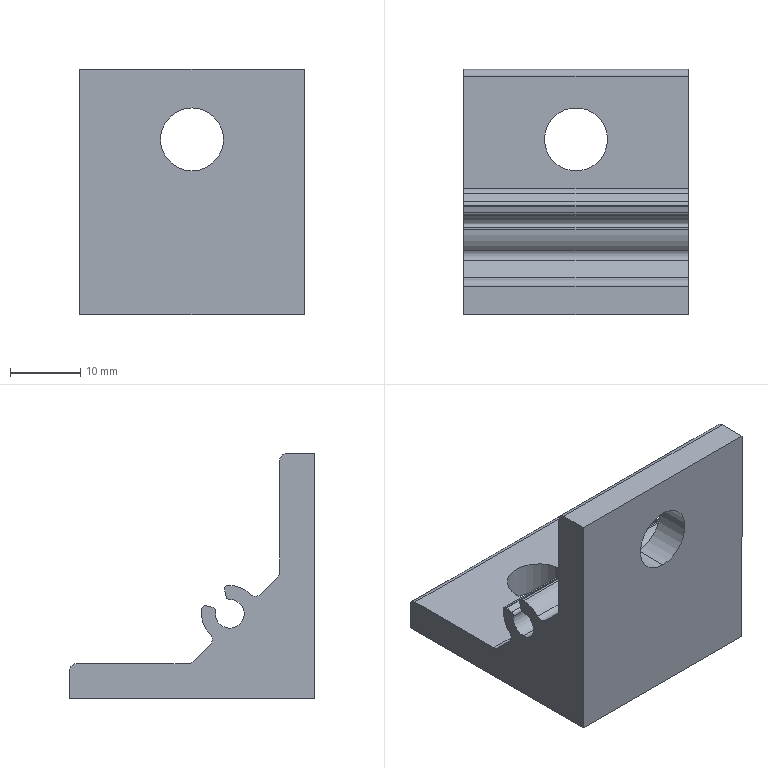Part | STEP file | HJLE-JJ90°-40_LE0724153021 | 1 solid | 33 faces | box 32 x 35 x 35 mm | volume 12807 mm3 | cylinder 21 | plane 12 | commonest cylinder face diameters 2 x6 1 x5 9 x4 4.1 x3 8.1 x3
STEP:
#1=CARTESIAN_POINT('',(0.,4.818,29.5));
#2=VERTEX_POINT('',#1);
#3=CARTESIAN_POINT('',(0.,4.818,20.5));
#4=VERTEX_POINT('',#3);
#5=CARTESIAN_POINT('',(0.,4.818,25.));
#6=DIRECTION('',(0.,-1.,0.));
#7=DIRECTION('',(0.,0.,-1.));
#8=AXIS2_PLACEMENT_3D('',#5,#6,#7);
#9=CIRCLE('',#8,4.5);
#10=EDGE_CURVE('',#2,#4,#9,.T.);
#11=ORIENTED_EDGE('',*,*,#10,.F.);
#12=CARTESIAN_POINT('',(0.,-0.182,29.5));
#13=VERTEX_POINT('',#12);
#14=CARTESIAN_POINT('',(0.,17.546,29.5));
#15=DIRECTION('',(0.,-1.,0.));
#16=VECTOR('',#15,1000.);
#17=LINE('',#14,#16);
#18=EDGE_CURVE('',#2,#13,#17,.T.);
#19=ORIENTED_EDGE('',*,*,#18,.T.);
#20=CARTESIAN_POINT('',(0.,-0.182,20.5));
#21=VERTEX_POINT('',#20);
#22=CARTESIAN_POINT('',(0.,-0.182,25.));
#23=DIRECTION('',(0.,-1.,0.));
#24=DIRECTION('',(0.,0.,-1.));
#25=AXIS2_PLACEMENT_3D('',#22,#23,#24);
#26=CIRCLE('',#25,4.5);
#27=EDGE_CURVE('',#13,#21,#26,.T.);
#28=ORIENTED_EDGE('',*,*,#27,.T.);
#29=CARTESIAN_POINT('',(0.,17.546,20.5));
#30=DIRECTION('',(0.,-1.,0.));
#31=VECTOR('',#30,1000.);
#32=LINE('',#29,#31);
#33=EDGE_CURVE('',#4,#21,#32,.T.);
#34=ORIENTED_EDGE('',*,*,#33,.F.);
#35=EDGE_LOOP('',(#11,#19,#28,#34));
#36=FACE_OUTER_BOUND('',#35,.T.);
#37=CARTESIAN_POINT('',(0.,17.546,25.));
#38=DIRECTION('',(0.,-1.,0.));
#39=DIRECTION('',(0.,0.,-1.));
#40=AXIS2_PLACEMENT_3D('',#37,#38,#39);
#41=CYLINDRICAL_SURFACE('',#40,4.5);
#42=ADVANCED_FACE('',(#36),#41,.F.);
#43=CARTESIAN_POINT('',(4.5,24.818,5.));
#44=VERTEX_POINT('',#43);
#45=CARTESIAN_POINT('',(-4.5,24.818,5.));
#46=VERTEX_POINT('',#45);
#47=CARTESIAN_POINT('',(0.,24.818,5.));
#48=DIRECTION('',(0.,0.,-1.));
#49=DIRECTION('',(-1.,0.,0.));
#50=AXIS2_PLACEMENT_3D('',#47,#48,#49);
#51=CIRCLE('',#50,4.5);
#52=EDGE_CURVE('',#44,#46,#51,.T.);
#53=ORIENTED_EDGE('',*,*,#52,.F.);
#54=CARTESIAN_POINT('',(4.5,24.818,0.));
#55=VERTEX_POINT('',#54);
#56=CARTESIAN_POINT('',(4.5,24.818,17.728));
#57=DIRECTION('',(0.,0.,-1.));
#58=VECTOR('',#57,1000.);
#59=LINE('',#56,#58);
#60=EDGE_CURVE('',#44,#55,#59,.T.);
#61=ORIENTED_EDGE('',*,*,#60,.T.);
#62=CARTESIAN_POINT('',(-4.5,24.818,0.));
#63=VERTEX_POINT('',#62);
#64=CARTESIAN_POINT('',(0.,24.818,0.));
#65=DIRECTION('',(0.,0.,-1.));
#66=DIRECTION('',(-1.,0.,0.));
#67=AXIS2_PLACEMENT_3D('',#64,#65,#66);
#68=CIRCLE('',#67,4.5);
#69=EDGE_CURVE('',#55,#63,#68,.T.);
#70=ORIENTED_EDGE('',*,*,#69,.T.);
#71=CARTESIAN_POINT('',(-4.5,24.818,17.728));
#72=DIRECTION('',(0.,0.,-1.));
#73=VECTOR('',#72,1000.);
#74=LINE('',#71,#73);
#75=EDGE_CURVE('',#46,#63,#74,.T.);
#76=ORIENTED_EDGE('',*,*,#75,.F.);
#77=EDGE_LOOP('',(#53,#61,#70,#76));
#78=FACE_OUTER_BOUND('',#77,.T.);
#79=CARTESIAN_POINT('',(0.,24.818,17.728));
#80=DIRECTION('',(0.,0.,-1.));
#81=DIRECTION('',(-1.,0.,0.));
#82=AXIS2_PLACEMENT_3D('',#79,#80,#81);
#83=CYLINDRICAL_SURFACE('',#82,4.5);
#84=ADVANCED_FACE('',(#78),#83,.F.);
#85=CARTESIAN_POINT('',(16.,11.922,10.054));
#86=VERTEX_POINT('',#85);
#87=CARTESIAN_POINT('',(16.,11.922,14.154));
#88=VERTEX_POINT('',#87);
#89=CARTESIAN_POINT('',(16.,11.922,12.104));
#90=DIRECTION('',(-1.,0.,0.));
#91=DIRECTION('',(0.,0.,1.));
#92=AXIS2_PLACEMENT_3D('',#89,#90,#91);
#93=CIRCLE('',#92,2.05);
#94=EDGE_CURVE('',#86,#88,#93,.T.);
#95=ORIENTED_EDGE('',*,*,#94,.F.);
#96=CARTESIAN_POINT('',(-16.,11.922,10.054));
#97=VERTEX_POINT('',#96);
#98=CARTESIAN_POINT('',(16.,11.922,10.054));
#99=DIRECTION('',(-1.,0.,0.));
#100=VECTOR('',#99,1000.);
#101=LINE('',#98,#100);
#102=EDGE_CURVE('',#86,#97,#101,.T.);
#103=ORIENTED_EDGE('',*,*,#102,.T.);
#104=CARTESIAN_POINT('',(-16.,11.922,14.154));
#105=VERTEX_POINT('',#104);
#106=CARTESIAN_POINT('',(-16.,11.922,12.104));
#107=DIRECTION('',(-1.,0.,0.));
#108=DIRECTION('',(0.,0.,1.));
#109=AXIS2_PLACEMENT_3D('',#106,#107,#108);
#110=CIRCLE('',#109,2.05);
#111=EDGE_CURVE('',#97,#105,#110,.T.);
#112=ORIENTED_EDGE('',*,*,#111,.T.);
#113=CARTESIAN_POINT('',(16.,11.922,14.154));
#114=DIRECTION('',(-1.,0.,0.));
#115=VECTOR('',#114,1000.);
#116=LINE('',#113,#115);
#117=EDGE_CURVE('',#88,#105,#116,.T.);
#118=ORIENTED_EDGE('',*,*,#117,.F.);
#119=EDGE_LOOP('',(#95,#103,#112,#118));
#120=FACE_OUTER_BOUND('',#119,.T.);
#121=CARTESIAN_POINT('',(16.,11.922,12.104));
#122=DIRECTION('',(-1.,0.,0.));
#123=DIRECTION('',(0.,0.,1.));
#124=AXIS2_PLACEMENT_3D('',#121,#122,#123);
#125=CYLINDRICAL_SURFACE('',#124,2.05);
#126=ADVANCED_FACE('',(#120),#125,.F.);
#127=CARTESIAN_POINT('',(16.,11.939,14.154));
#128=VERTEX_POINT('',#127);
#129=CARTESIAN_POINT('',(16.,11.922,12.104));
#130=DIRECTION('',(-1.,0.,0.));
#131=DIRECTION('',(0.,0.,1.));
#132=AXIS2_PLACEMENT_3D('',#129,#130,#131);
#133=CIRCLE('',#132,2.05);
#134=EDGE_CURVE('',#88,#128,#133,.T.);
#135=ORIENTED_EDGE('',*,*,#134,.F.);
#136=ORIENTED_EDGE('',*,*,#117,.T.);
#137=CARTESIAN_POINT('',(-16.,11.939,14.154));
#138=VERTEX_POINT('',#137);
#139=CARTESIAN_POINT('',(-16.,11.922,12.104));
#140=DIRECTION('',(-1.,0.,0.));
#141=DIRECTION('',(0.,0.,1.));
#142=AXIS2_PLACEMENT_3D('',#139,#140,#141);
#143=CIRCLE('',#142,2.05);
#144=EDGE_CURVE('',#105,#138,#143,.T.);
#145=ORIENTED_EDGE('',*,*,#144,.T.);
#146=CARTESIAN_POINT('',(16.,11.939,14.154));
#147=DIRECTION('',(-1.,0.,0.));
#148=VECTOR('',#147,1000.);
#149=LINE('',#146,#148);
#150=EDGE_CURVE('',#128,#138,#149,.T.);
#151=ORIENTED_EDGE('',*,*,#150,.F.);
#152=EDGE_LOOP('',(#135,#136,#145,#151));
#153=FACE_OUTER_BOUND('',#152,.T.);
#154=CARTESIAN_POINT('',(16.,11.922,12.104));
#155=DIRECTION('',(-1.,0.,0.));
#156=DIRECTION('',(0.,0.,1.));
#157=AXIS2_PLACEMENT_3D('',#154,#155,#156);
#158=CYLINDRICAL_SURFACE('',#157,2.05);
#159=ADVANCED_FACE('',(#153),#158,.F.);
#160=CARTESIAN_POINT('',(16.,11.922,16.154));
#161=VERTEX_POINT('',#160);
#162=CARTESIAN_POINT('',(16.,8.999,14.907));
#163=VERTEX_POINT('',#162);
#164=CARTESIAN_POINT('',(16.,11.922,12.104));
#165=DIRECTION('',(1.,0.,0.));
#166=DIRECTION('',(0.,0.,1.));
#167=AXIS2_PLACEMENT_3D('',#164,#165,#166);
#168=CIRCLE('',#167,4.05);
#169=EDGE_CURVE('',#161,#163,#168,.T.);
#170=ORIENTED_EDGE('',*,*,#169,.F.);
#171=CARTESIAN_POINT('',(-16.,11.922,16.154));
#172=VERTEX_POINT('',#171);
#173=CARTESIAN_POINT('',(16.,11.922,16.154));
#174=DIRECTION('',(-1.,0.,0.));
#175=VECTOR('',#174,1000.);
#176=LINE('',#173,#175);
#177=EDGE_CURVE('',#161,#172,#176,.T.);
#178=ORIENTED_EDGE('',*,*,#177,.T.);
#179=CARTESIAN_POINT('',(-16.,8.999,14.907));
#180=VERTEX_POINT('',#179);
#181=CARTESIAN_POINT('',(-16.,11.922,12.104));
#182=DIRECTION('',(1.,0.,0.));
#183=DIRECTION('',(0.,0.,1.));
#184=AXIS2_PLACEMENT_3D('',#181,#182,#183);
#185=CIRCLE('',#184,4.05);
#186=EDGE_CURVE('',#172,#180,#185,.T.);
#187=ORIENTED_EDGE('',*,*,#186,.T.);
#188=CARTESIAN_POINT('',(16.,8.999,14.907));
#189=DIRECTION('',(1.,0.,0.));
#190=VECTOR('',#189,1000.);
#191=LINE('',#188,#190);
#192=EDGE_CURVE('',#180,#163,#191,.T.);
#193=ORIENTED_EDGE('',*,*,#192,.T.);
#194=EDGE_LOOP('',(#170,#178,#187,#193));
#195=FACE_OUTER_BOUND('',#194,.T.);
#196=CARTESIAN_POINT('',(16.,11.922,12.104));
#197=DIRECTION('',(-1.,0.,0.));
#198=DIRECTION('',(0.,0.,1.));
#199=AXIS2_PLACEMENT_3D('',#196,#197,#198);
#200=CYLINDRICAL_SURFACE('',#199,4.05);
#201=ADVANCED_FACE('',(#195),#200,.T.);
#202=CARTESIAN_POINT('',(16.,15.278,13.252));
#203=VERTEX_POINT('',#202);
#204=CARTESIAN_POINT('',(16.,15.409,13.27));
#205=VERTEX_POINT('',#204);
#206=CARTESIAN_POINT('',(16.,15.409,12.77));
#207=DIRECTION('',(-1.,0.,0.));
#208=DIRECTION('',(0.,0.,1.));
#209=AXIS2_PLACEMENT_3D('',#206,#207,#208);
#210=CIRCLE('',#209,0.5);
#211=EDGE_CURVE('',#203,#205,#210,.T.);
#212=ORIENTED_EDGE('',*,*,#211,.T.);
#213=CARTESIAN_POINT('',(-16.,15.409,13.27));
#214=VERTEX_POINT('',#213);
#215=CARTESIAN_POINT('',(16.,15.409,13.27));
#216=DIRECTION('',(-1.,0.,0.));
#217=VECTOR('',#216,1000.);
#218=LINE('',#215,#217);
#219=EDGE_CURVE('',#205,#214,#218,.T.);
#220=ORIENTED_EDGE('',*,*,#219,.T.);
#221=CARTESIAN_POINT('',(-16.,15.278,13.252));
#222=VERTEX_POINT('',#221);
#223=CARTESIAN_POINT('',(-16.,15.409,12.77));
#224=DIRECTION('',(1.,0.,0.));
#225=DIRECTION('',(0.,0.,1.));
#226=AXIS2_PLACEMENT_3D('',#223,#224,#225);
#227=CIRCLE('',#226,0.5);
#228=EDGE_CURVE('',#214,#222,#227,.T.);
#229=ORIENTED_EDGE('',*,*,#228,.T.);
#230=CARTESIAN_POINT('',(16.,15.278,13.252));
#231=DIRECTION('',(1.,0.,0.));
#232=VECTOR('',#231,1000.);
#233=LINE('',#230,#232);
#234=EDGE_CURVE('',#222,#203,#233,.T.);
#235=ORIENTED_EDGE('',*,*,#234,.T.);
#236=EDGE_LOOP('',(#212,#220,#229,#235));
#237=FACE_OUTER_BOUND('',#236,.T.);
#238=CARTESIAN_POINT('',(16.,15.409,12.77));
#239=DIRECTION('',(-1.,0.,0.));
#240=DIRECTION('',(0.,0.,1.));
#241=AXIS2_PLACEMENT_3D('',#238,#239,#240);
#242=CYLINDRICAL_SURFACE('',#241,0.5);
#243=ADVANCED_FACE('',(#237),#242,.T.);
#244=CARTESIAN_POINT('',(0.,-0.182,25.));
#245=DIRECTION('',(0.,-1.,0.));
#246=DIRECTION('',(0.,0.,-1.));
#247=AXIS2_PLACEMENT_3D('',#244,#245,#246);
#248=CIRCLE('',#247,4.5);
#249=EDGE_CURVE('',#21,#13,#248,.T.);
#250=ORIENTED_EDGE('',*,*,#249,.F.);
#251=ORIENTED_EDGE('',*,*,#27,.F.);
#252=EDGE_LOOP('',(#250,#251));
#253=FACE_BOUND('',#252,.T.);
#254=CARTESIAN_POINT('',(16.,-0.182,35.));
#255=VERTEX_POINT('',#254);
#256=CARTESIAN_POINT('',(16.,-0.182,0.));
#257=VERTEX_POINT('',#256);
#258=CARTESIAN_POINT('',(16.,-0.182,0.));
#259=DIRECTION('',(0.,0.,-1.));
#260=VECTOR('',#259,1000.);
#261=LINE('',#258,#260);
#262=EDGE_CURVE('',#255,#257,#261,.T.);
#263=ORIENTED_EDGE('',*,*,#262,.F.);
#264=CARTESIAN_POINT('',(-16.,-0.182,35.));
#265=VERTEX_POINT('',#264);
#266=CARTESIAN_POINT('',(16.,-0.182,35.));
#267=DIRECTION('',(1.,0.,0.));
#268=VECTOR('',#267,1000.);
#269=LINE('',#266,#268);
#270=EDGE_CURVE('',#265,#255,#269,.T.);
#271=ORIENTED_EDGE('',*,*,#270,.F.);
#272=CARTESIAN_POINT('',(-16.,-0.182,0.));
#273=VERTEX_POINT('',#272);
#274=CARTESIAN_POINT('',(-16.,-0.182,0.));
#275=DIRECTION('',(0.,0.,1.));
#276=VECTOR('',#275,1000.);
#277=LINE('',#274,#276);
#278=EDGE_CURVE('',#273,#265,#277,.T.);
#279=ORIENTED_EDGE('',*,*,#278,.F.);
#280=CARTESIAN_POINT('',(16.,-0.182,0.));
#281=DIRECTION('',(-1.,0.,0.));
#282=VECTOR('',#281,1000.);
#283=LINE('',#280,#282);
#284=EDGE_CURVE('',#257,#273,#283,.T.);
#285=ORIENTED_EDGE('',*,*,#284,.F.);
#286=EDGE_LOOP('',(#263,#271,#279,#285));
#287=FACE_OUTER_BOUND('',#286,.T.);
#288=CARTESIAN_POINT('',(16.,-0.182,0.));
#289=DIRECTION('',(0.,1.,0.));
#290=DIRECTION('',(0.,0.,1.));
#291=AXIS2_PLACEMENT_3D('',#288,#289,#290);
#292=PLANE('',#291);
#293=ADVANCED_FACE('',(#253,#287),#292,.F.);
#294=ORIENTED_EDGE('',*,*,#18,.F.);
#295=CARTESIAN_POINT('',(0.,4.818,25.));
#296=DIRECTION('',(0.,-1.,0.));
#297=DIRECTION('',(0.,0.,-1.));
#298=AXIS2_PLACEMENT_3D('',#295,#296,#297);
#299=CIRCLE('',#298,4.5);
#300=EDGE_CURVE('',#4,#2,#299,.T.);
#301=ORIENTED_EDGE('',*,*,#300,.F.);
#302=ORIENTED_EDGE('',*,*,#33,.T.);
#303=ORIENTED_EDGE('',*,*,#249,.T.);
#304=EDGE_LOOP('',(#294,#301,#302,#303));
#305=FACE_OUTER_BOUND('',#304,.T.);
#306=CARTESIAN_POINT('',(0.,17.546,25.));
#307=DIRECTION('',(0.,-1.,0.));
#308=DIRECTION('',(0.,0.,-1.));
#309=AXIS2_PLACEMENT_3D('',#306,#307,#308);
#310=CYLINDRICAL_SURFACE('',#309,4.5);
#311=ADVANCED_FACE('',(#305),#310,.F.);
#312=CARTESIAN_POINT('',(0.,24.818,0.));
#313=DIRECTION('',(0.,0.,-1.));
#314=DIRECTION('',(-1.,0.,0.));
#315=AXIS2_PLACEMENT_3D('',#312,#313,#314);
#316=CIRCLE('',#315,4.5);
#317=EDGE_CURVE('',#63,#55,#316,.T.);
#318=ORIENTED_EDGE('',*,*,#317,.F.);
#319=ORIENTED_EDGE('',*,*,#69,.F.);
#320=EDGE_LOOP('',(#318,#319));
#321=FACE_BOUND('',#320,.T.);
#322=CARTESIAN_POINT('',(16.,34.818,0.));
#323=VERTEX_POINT('',#322);
#324=CARTESIAN_POINT('',(16.,-0.182,0.));
#325=DIRECTION('',(0.,1.,0.));
#326=VECTOR('',#325,1000.);
#327=LINE('',#324,#326);
#328=EDGE_CURVE('',#257,#323,#327,.T.);
#329=ORIENTED_EDGE('',*,*,#328,.F.);
#330=ORIENTED_EDGE('',*,*,#284,.T.);
#331=CARTESIAN_POINT('',(-16.,34.818,0.));
#332=VERTEX_POINT('',#331);
#333=CARTESIAN_POINT('',(-16.,-0.182,0.));
#334=DIRECTION('',(0.,-1.,0.));
#335=VECTOR('',#334,1000.);
#336=LINE('',#333,#335);
#337=EDGE_CURVE('',#332,#273,#336,.T.);
#338=ORIENTED_EDGE('',*,*,#337,.F.);
#339=CARTESIAN_POINT('',(16.,34.818,0.));
#340=DIRECTION('',(-1.,0.,0.));
#341=VECTOR('',#340,1000.);
#342=LINE('',#339,#341);
#343=EDGE_CURVE('',#323,#332,#342,.T.);
#344=ORIENTED_EDGE('',*,*,#343,.F.);
#345=EDGE_LOOP('',(#329,#330,#338,#344));
#346=FACE_OUTER_BOUND('',#345,.T.);
#347=CARTESIAN_POINT('',(16.,-0.182,0.));
#348=DIRECTION('',(0.,0.,1.));
#349=DIRECTION('',(1.,0.,0.));
#350=AXIS2_PLACEMENT_3D('',#347,#348,#349);
#351=PLANE('',#350);
#352=ADVANCED_FACE('',(#321,#346),#351,.F.);
#353=CARTESIAN_POINT('',(16.,13.947,12.428));
#354=VERTEX_POINT('',#353);
#355=CARTESIAN_POINT('',(16.,11.922,12.104));
#356=DIRECTION('',(-1.,0.,0.));
#357=DIRECTION('',(0.,0.,1.));
#358=AXIS2_PLACEMENT_3D('',#355,#356,#357);
#359=CIRCLE('',#358,2.05);
#360=EDGE_CURVE('',#354,#86,#359,.T.);
#361=ORIENTED_EDGE('',*,*,#360,.T.);
#362=ORIENTED_EDGE('',*,*,#94,.T.);
#363=ORIENTED_EDGE('',*,*,#134,.T.);
#364=CARTESIAN_POINT('',(16.,12.425,14.522));
#365=VERTEX_POINT('',#364);
#366=CARTESIAN_POINT('',(16.,11.943,14.654));
#367=DIRECTION('',(-1.,0.,0.));
#368=DIRECTION('',(0.,0.,1.));
#369=AXIS2_PLACEMENT_3D('',#366,#367,#368);
#370=CIRCLE('',#369,0.5);
#371=EDGE_CURVE('',#365,#128,#370,.T.);
#372=ORIENTED_EDGE('',*,*,#371,.F.);
#373=CARTESIAN_POINT('',(16.,12.697,15.51));
#374=VERTEX_POINT('',#373);
#375=CARTESIAN_POINT('',(16.,12.697,15.51));
#376=DIRECTION('',(0.,0.2648,0.9643));
#377=VECTOR('',#376,1000.);
#378=LINE('',#375,#377);
#379=EDGE_CURVE('',#365,#374,#378,.T.);
#380=ORIENTED_EDGE('',*,*,#379,.T.);
#381=CARTESIAN_POINT('',(16.,12.256,16.14));
#382=VERTEX_POINT('',#381);
#383=CARTESIAN_POINT('',(16.,12.215,15.642));
#384=DIRECTION('',(-1.,0.,0.));
#385=DIRECTION('',(0.,0.,1.));
#386=AXIS2_PLACEMENT_3D('',#383,#384,#385);
#387=CIRCLE('',#386,0.5);
#388=EDGE_CURVE('',#382,#374,#387,.T.);
#389=ORIENTED_EDGE('',*,*,#388,.F.);
#390=CARTESIAN_POINT('',(16.,11.922,12.104));
#391=DIRECTION('',(1.,0.,0.));
#392=DIRECTION('',(0.,0.,1.));
#393=AXIS2_PLACEMENT_3D('',#390,#391,#392);
#394=CIRCLE('',#393,4.05);
#395=EDGE_CURVE('',#382,#161,#394,.T.);
#396=ORIENTED_EDGE('',*,*,#395,.T.);
#397=ORIENTED_EDGE('',*,*,#169,.T.);
#398=CARTESIAN_POINT('',(16.,7.57,14.892));
#399=VERTEX_POINT('',#398);
#400=CARTESIAN_POINT('',(16.,8.277,15.599));
#401=DIRECTION('',(-1.,0.,0.));
#402=DIRECTION('',(0.,0.,1.));
#403=AXIS2_PLACEMENT_3D('',#400,#401,#402);
#404=CIRCLE('',#403,1.);
#405=EDGE_CURVE('',#163,#399,#404,.T.);
#406=ORIENTED_EDGE('',*,*,#405,.T.);
#407=CARTESIAN_POINT('',(16.,5.111,17.351));
#408=VERTEX_POINT('',#407);
#409=CARTESIAN_POINT('',(16.,7.57,14.892));
#410=DIRECTION('',(0.,-0.7071,0.7071));
#411=VECTOR('',#410,1000.);
#412=LINE('',#409,#411);
#413=EDGE_CURVE('',#399,#408,#412,.T.);
#414=ORIENTED_EDGE('',*,*,#413,.T.);
#415=CARTESIAN_POINT('',(16.,4.818,18.058));
#416=VERTEX_POINT('',#415);
#417=CARTESIAN_POINT('',(16.,5.818,18.058));
#418=DIRECTION('',(-1.,0.,0.));
#419=DIRECTION('',(0.,0.,1.));
#420=AXIS2_PLACEMENT_3D('',#417,#418,#419);
#421=CIRCLE('',#420,1.);
#422=EDGE_CURVE('',#408,#416,#421,.T.);
#423=ORIENTED_EDGE('',*,*,#422,.T.);
#424=CARTESIAN_POINT('',(16.,4.818,34.));
#425=VERTEX_POINT('',#424);
#426=CARTESIAN_POINT('',(16.,4.818,15.642));
#427=DIRECTION('',(0.,0.,1.));
#428=VECTOR('',#427,1000.);
#429=LINE('',#426,#428);
#430=EDGE_CURVE('',#416,#425,#429,.T.);
#431=ORIENTED_EDGE('',*,*,#430,.T.);
#432=CARTESIAN_POINT('',(16.,3.818,35.));
#433=VERTEX_POINT('',#432);
#434=CARTESIAN_POINT('',(16.,3.818,34.));
#435=DIRECTION('',(-1.,0.,0.));
#436=DIRECTION('',(0.,0.,1.));
#437=AXIS2_PLACEMENT_3D('',#434,#435,#436);
#438=CIRCLE('',#437,1.);
#439=EDGE_CURVE('',#433,#425,#438,.T.);
#440=ORIENTED_EDGE('',*,*,#439,.F.);
#441=CARTESIAN_POINT('',(16.,12.215,35.));
#442=DIRECTION('',(0.,-1.,0.));
#443=VECTOR('',#442,1000.);
#444=LINE('',#441,#443);
#445=EDGE_CURVE('',#433,#255,#444,.T.);
#446=ORIENTED_EDGE('',*,*,#445,.T.);
#447=ORIENTED_EDGE('',*,*,#262,.T.);
#448=ORIENTED_EDGE('',*,*,#328,.T.);
#449=CARTESIAN_POINT('',(16.,34.818,4.));
#450=VERTEX_POINT('',#449);
#451=CARTESIAN_POINT('',(16.,34.818,15.642));
#452=DIRECTION('',(0.,0.,1.));
#453=VECTOR('',#452,1000.);
#454=LINE('',#451,#453);
#455=EDGE_CURVE('',#323,#450,#454,.T.);
#456=ORIENTED_EDGE('',*,*,#455,.T.);
#457=CARTESIAN_POINT('',(16.,33.818,5.));
#458=VERTEX_POINT('',#457);
#459=CARTESIAN_POINT('',(16.,33.818,4.));
#460=DIRECTION('',(-1.,0.,0.));
#461=DIRECTION('',(0.,0.,1.));
#462=AXIS2_PLACEMENT_3D('',#459,#460,#461);
#463=CIRCLE('',#462,1.);
#464=EDGE_CURVE('',#458,#450,#463,.T.);
#465=ORIENTED_EDGE('',*,*,#464,.F.);
#466=CARTESIAN_POINT('',(16.,17.876,5.));
#467=VERTEX_POINT('',#466);
#468=CARTESIAN_POINT('',(16.,12.215,5.));
#469=DIRECTION('',(0.,-1.,0.));
#470=VECTOR('',#469,1000.);
#471=LINE('',#468,#470);
#472=EDGE_CURVE('',#458,#467,#471,.T.);
#473=ORIENTED_EDGE('',*,*,#472,.T.);
#474=CARTESIAN_POINT('',(16.,17.169,5.293));
#475=VERTEX_POINT('',#474);
#476=CARTESIAN_POINT('',(16.,17.876,6.));
#477=DIRECTION('',(-1.,0.,0.));
#478=DIRECTION('',(0.,0.,1.));
#479=AXIS2_PLACEMENT_3D('',#476,#477,#478);
#480=CIRCLE('',#479,1.);
#481=EDGE_CURVE('',#467,#475,#480,.T.);
#482=ORIENTED_EDGE('',*,*,#481,.T.);
#483=CARTESIAN_POINT('',(16.,14.71,7.752));
#484=VERTEX_POINT('',#483);
#485=CARTESIAN_POINT('',(16.,17.169,5.293));
#486=DIRECTION('',(0.,-0.7071,0.7071));
#487=VECTOR('',#486,1000.);
#488=LINE('',#485,#487);
#489=EDGE_CURVE('',#475,#484,#488,.T.);
#490=ORIENTED_EDGE('',*,*,#489,.T.);
#491=CARTESIAN_POINT('',(16.,14.725,9.181));
#492=VERTEX_POINT('',#491);
#493=CARTESIAN_POINT('',(16.,15.417,8.459));
#494=DIRECTION('',(-1.,0.,0.));
#495=DIRECTION('',(0.,0.,1.));
#496=AXIS2_PLACEMENT_3D('',#493,#494,#495);
#497=CIRCLE('',#496,1.);
#498=EDGE_CURVE('',#484,#492,#497,.T.);
#499=ORIENTED_EDGE('',*,*,#498,.T.);
#500=CARTESIAN_POINT('',(16.,15.9,12.863));
#501=VERTEX_POINT('',#500);
#502=CARTESIAN_POINT('',(16.,11.922,12.104));
#503=DIRECTION('',(1.,0.,0.));
#504=DIRECTION('',(0.,0.,1.));
#505=AXIS2_PLACEMENT_3D('',#502,#503,#504);
#506=CIRCLE('',#505,4.05);
#507=EDGE_CURVE('',#492,#501,#506,.T.);
#508=ORIENTED_EDGE('',*,*,#507,.T.);
#509=CARTESIAN_POINT('',(16.,15.409,12.77));
#510=DIRECTION('',(-1.,0.,0.));
#511=DIRECTION('',(0.,0.,1.));
#512=AXIS2_PLACEMENT_3D('',#509,#510,#511);
#513=CIRCLE('',#512,0.5);
#514=EDGE_CURVE('',#205,#501,#513,.T.);
#515=ORIENTED_EDGE('',*,*,#514,.F.);
#516=ORIENTED_EDGE('',*,*,#211,.F.);
#517=CARTESIAN_POINT('',(16.,14.309,12.989));
#518=VERTEX_POINT('',#517);
#519=CARTESIAN_POINT('',(16.,15.278,13.252));
#520=DIRECTION('',(0.,-0.9651,-0.2617));
#521=VECTOR('',#520,1000.);
#522=LINE('',#519,#521);
#523=EDGE_CURVE('',#203,#518,#522,.T.);
#524=ORIENTED_EDGE('',*,*,#523,.T.);
#525=CARTESIAN_POINT('',(16.,14.44,12.507));
#526=DIRECTION('',(-1.,0.,0.));
#527=DIRECTION('',(0.,0.,1.));
#528=AXIS2_PLACEMENT_3D('',#525,#526,#527);
#529=CIRCLE('',#528,0.5);
#530=EDGE_CURVE('',#354,#518,#529,.T.);
#531=ORIENTED_EDGE('',*,*,#530,.F.);
#532=EDGE_LOOP('',(#361,#362,#363,#372,#380,#389,#396,#397,#406,#414,#423,#431,#440,#446,#447,#448,#456,#465,#473,#482,#490,#499,#508,#515,#516,#524,#531));
#533=FACE_OUTER_BOUND('',#532,.T.);
#534=CARTESIAN_POINT('',(16.,12.215,15.642));
#535=DIRECTION('',(1.,0.,0.));
#536=DIRECTION('',(0.,0.,-1.));
#537=AXIS2_PLACEMENT_3D('',#534,#535,#536);
#538=PLANE('',#537);
#539=ADVANCED_FACE('',(#533),#538,.T.);
#540=ORIENTED_EDGE('',*,*,#445,.F.);
#541=CARTESIAN_POINT('',(-16.,3.818,35.));
#542=VERTEX_POINT('',#541);
#543=CARTESIAN_POINT('',(16.,3.818,35.));
#544=DIRECTION('',(1.,0.,0.));
#545=VECTOR('',#544,1000.);
#546=LINE('',#543,#545);
#547=EDGE_CURVE('',#542,#433,#546,.T.);
#548=ORIENTED_EDGE('',*,*,#547,.F.);
#549=CARTESIAN_POINT('',(-16.,-0.182,35.));
#550=DIRECTION('',(0.,1.,0.));
#551=VECTOR('',#550,1000.);
#552=LINE('',#549,#551);
#553=EDGE_CURVE('',#265,#542,#552,.T.);
#554=ORIENTED_EDGE('',*,*,#553,.F.);
#555=ORIENTED_EDGE('',*,*,#270,.T.);
#556=EDGE_LOOP('',(#540,#548,#554,#555));
#557=FACE_OUTER_BOUND('',#556,.T.);
#558=CARTESIAN_POINT('',(16.,-0.182,35.));
#559=DIRECTION('',(0.,0.,-1.));
#560=DIRECTION('',(-1.,0.,0.));
#561=AXIS2_PLACEMENT_3D('',#558,#559,#560);
#562=PLANE('',#561);
#563=ADVANCED_FACE('',(#557),#562,.F.);
#564=CARTESIAN_POINT('',(-16.,12.425,14.522));
#565=VERTEX_POINT('',#564);
#566=CARTESIAN_POINT('',(-16.,11.943,14.654));
#567=DIRECTION('',(1.,0.,0.));
#568=DIRECTION('',(0.,0.,1.));
#569=AXIS2_PLACEMENT_3D('',#566,#567,#568);
#570=CIRCLE('',#569,0.5);
#571=EDGE_CURVE('',#138,#565,#570,.T.);
#572=ORIENTED_EDGE('',*,*,#571,.F.);
#573=ORIENTED_EDGE('',*,*,#144,.F.);
#574=ORIENTED_EDGE('',*,*,#111,.F.);
#575=CARTESIAN_POINT('',(-16.,13.947,12.428));
#576=VERTEX_POINT('',#575);
#577=CARTESIAN_POINT('',(-16.,11.922,12.104));
#578=DIRECTION('',(-1.,0.,0.));
#579=DIRECTION('',(0.,0.,1.));
#580=AXIS2_PLACEMENT_3D('',#577,#578,#579);
#581=CIRCLE('',#580,2.05);
#582=EDGE_CURVE('',#576,#97,#581,.T.);
#583=ORIENTED_EDGE('',*,*,#582,.F.);
#584=CARTESIAN_POINT('',(-16.,14.309,12.989));
#585=VERTEX_POINT('',#584);
#586=CARTESIAN_POINT('',(-16.,14.44,12.507));
#587=DIRECTION('',(1.,0.,0.));
#588=DIRECTION('',(0.,0.,1.));
#589=AXIS2_PLACEMENT_3D('',#586,#587,#588);
#590=CIRCLE('',#589,0.5);
#591=EDGE_CURVE('',#585,#576,#590,.T.);
#592=ORIENTED_EDGE('',*,*,#591,.F.);
#593=CARTESIAN_POINT('',(-16.,15.278,13.252));
#594=DIRECTION('',(0.,0.9651,0.2617));
#595=VECTOR('',#594,1000.);
#596=LINE('',#593,#595);
#597=EDGE_CURVE('',#585,#222,#596,.T.);
#598=ORIENTED_EDGE('',*,*,#597,.T.);
#599=ORIENTED_EDGE('',*,*,#228,.F.);
#600=CARTESIAN_POINT('',(-16.,15.9,12.863));
#601=VERTEX_POINT('',#600);
#602=CARTESIAN_POINT('',(-16.,15.409,12.77));
#603=DIRECTION('',(1.,0.,0.));
#604=DIRECTION('',(0.,0.,1.));
#605=AXIS2_PLACEMENT_3D('',#602,#603,#604);
#606=CIRCLE('',#605,0.5);
#607=EDGE_CURVE('',#601,#214,#606,.T.);
#608=ORIENTED_EDGE('',*,*,#607,.F.);
#609=CARTESIAN_POINT('',(-16.,14.725,9.181));
#610=VERTEX_POINT('',#609);
#611=CARTESIAN_POINT('',(-16.,11.922,12.104));
#612=DIRECTION('',(1.,0.,0.));
#613=DIRECTION('',(0.,0.,1.));
#614=AXIS2_PLACEMENT_3D('',#611,#612,#613);
#615=CIRCLE('',#614,4.05);
#616=EDGE_CURVE('',#610,#601,#615,.T.);
#617=ORIENTED_EDGE('',*,*,#616,.F.);
#618=CARTESIAN_POINT('',(-16.,14.71,7.752));
#619=VERTEX_POINT('',#618);
#620=CARTESIAN_POINT('',(-16.,15.417,8.459));
#621=DIRECTION('',(1.,0.,0.));
#622=DIRECTION('',(0.,0.,1.));
#623=AXIS2_PLACEMENT_3D('',#620,#621,#622);
#624=CIRCLE('',#623,1.);
#625=EDGE_CURVE('',#610,#619,#624,.T.);
#626=ORIENTED_EDGE('',*,*,#625,.T.);
#627=CARTESIAN_POINT('',(-16.,17.169,5.293));
#628=VERTEX_POINT('',#627);
#629=CARTESIAN_POINT('',(-16.,17.169,5.293));
#630=DIRECTION('',(0.,-0.7071,0.7071));
#631=VECTOR('',#630,1000.);
#632=LINE('',#629,#631);
#633=EDGE_CURVE('',#628,#619,#632,.T.);
#634=ORIENTED_EDGE('',*,*,#633,.F.);
#635=CARTESIAN_POINT('',(-16.,17.876,5.));
#636=VERTEX_POINT('',#635);
#637=CARTESIAN_POINT('',(-16.,17.876,6.));
#638=DIRECTION('',(1.,0.,0.));
#639=DIRECTION('',(0.,0.,1.));
#640=AXIS2_PLACEMENT_3D('',#637,#638,#639);
#641=CIRCLE('',#640,1.);
#642=EDGE_CURVE('',#628,#636,#641,.T.);
#643=ORIENTED_EDGE('',*,*,#642,.T.);
#644=CARTESIAN_POINT('',(-16.,33.818,5.));
#645=VERTEX_POINT('',#644);
#646=CARTESIAN_POINT('',(-16.,12.215,5.));
#647=DIRECTION('',(0.,-1.,0.));
#648=VECTOR('',#647,1000.);
#649=LINE('',#646,#648);
#650=EDGE_CURVE('',#645,#636,#649,.T.);
#651=ORIENTED_EDGE('',*,*,#650,.F.);
#652=CARTESIAN_POINT('',(-16.,34.818,4.));
#653=VERTEX_POINT('',#652);
#654=CARTESIAN_POINT('',(-16.,33.818,4.));
#655=DIRECTION('',(1.,0.,0.));
#656=DIRECTION('',(0.,0.,1.));
#657=AXIS2_PLACEMENT_3D('',#654,#655,#656);
#658=CIRCLE('',#657,1.);
#659=EDGE_CURVE('',#653,#645,#658,.T.);
#660=ORIENTED_EDGE('',*,*,#659,.F.);
#661=CARTESIAN_POINT('',(-16.,34.818,15.642));
#662=DIRECTION('',(0.,0.,1.));
#663=VECTOR('',#662,1000.);
#664=LINE('',#661,#663);
#665=EDGE_CURVE('',#332,#653,#664,.T.);
#666=ORIENTED_EDGE('',*,*,#665,.F.);
#667=ORIENTED_EDGE('',*,*,#337,.T.);
#668=ORIENTED_EDGE('',*,*,#278,.T.);
#669=ORIENTED_EDGE('',*,*,#553,.T.);
#670=CARTESIAN_POINT('',(-16.,4.818,34.));
#671=VERTEX_POINT('',#670);
#672=CARTESIAN_POINT('',(-16.,3.818,34.));
#673=DIRECTION('',(1.,0.,0.));
#674=DIRECTION('',(0.,0.,1.));
#675=AXIS2_PLACEMENT_3D('',#672,#673,#674);
#676=CIRCLE('',#675,1.);
#677=EDGE_CURVE('',#671,#542,#676,.T.);
#678=ORIENTED_EDGE('',*,*,#677,.F.);
#679=CARTESIAN_POINT('',(-16.,4.818,18.058));
#680=VERTEX_POINT('',#679);
#681=CARTESIAN_POINT('',(-16.,4.818,15.642));
#682=DIRECTION('',(0.,0.,1.));
#683=VECTOR('',#682,1000.);
#684=LINE('',#681,#683);
#685=EDGE_CURVE('',#680,#671,#684,.T.);
#686=ORIENTED_EDGE('',*,*,#685,.F.);
#687=CARTESIAN_POINT('',(-16.,5.111,17.351));
#688=VERTEX_POINT('',#687);
#689=CARTESIAN_POINT('',(-16.,5.818,18.058));
#690=DIRECTION('',(1.,0.,0.));
#691=DIRECTION('',(0.,0.,1.));
#692=AXIS2_PLACEMENT_3D('',#689,#690,#691);
#693=CIRCLE('',#692,1.);
#694=EDGE_CURVE('',#680,#688,#693,.T.);
#695=ORIENTED_EDGE('',*,*,#694,.T.);
#696=CARTESIAN_POINT('',(-16.,7.57,14.892));
#697=VERTEX_POINT('',#696);
#698=CARTESIAN_POINT('',(-16.,7.57,14.892));
#699=DIRECTION('',(0.,-0.7071,0.7071));
#700=VECTOR('',#699,1000.);
#701=LINE('',#698,#700);
#702=EDGE_CURVE('',#697,#688,#701,.T.);
#703=ORIENTED_EDGE('',*,*,#702,.F.);
#704=CARTESIAN_POINT('',(-16.,8.277,15.599));
#705=DIRECTION('',(1.,0.,0.));
#706=DIRECTION('',(0.,0.,1.));
#707=AXIS2_PLACEMENT_3D('',#704,#705,#706);
#708=CIRCLE('',#707,1.);
#709=EDGE_CURVE('',#697,#180,#708,.T.);
#710=ORIENTED_EDGE('',*,*,#709,.T.);
#711=ORIENTED_EDGE('',*,*,#186,.F.);
#712=CARTESIAN_POINT('',(-16.,12.256,16.14));
#713=VERTEX_POINT('',#712);
#714=CARTESIAN_POINT('',(-16.,11.922,12.104));
#715=DIRECTION('',(1.,0.,0.));
#716=DIRECTION('',(0.,0.,1.));
#717=AXIS2_PLACEMENT_3D('',#714,#715,#716);
#718=CIRCLE('',#717,4.05);
#719=EDGE_CURVE('',#713,#172,#718,.T.);
#720=ORIENTED_EDGE('',*,*,#719,.F.);
#721=CARTESIAN_POINT('',(-16.,12.697,15.51));
#722=VERTEX_POINT('',#721);
#723=CARTESIAN_POINT('',(-16.,12.215,15.642));
#724=DIRECTION('',(1.,0.,0.));
#725=DIRECTION('',(0.,0.,1.));
#726=AXIS2_PLACEMENT_3D('',#723,#724,#725);
#727=CIRCLE('',#726,0.5);
#728=EDGE_CURVE('',#722,#713,#727,.T.);
#729=ORIENTED_EDGE('',*,*,#728,.F.);
#730=CARTESIAN_POINT('',(-16.,12.697,15.51));
#731=DIRECTION('',(0.,-0.2648,-0.9643));
#732=VECTOR('',#731,1000.);
#733=LINE('',#730,#732);
#734=EDGE_CURVE('',#722,#565,#733,.T.);
#735=ORIENTED_EDGE('',*,*,#734,.T.);
#736=EDGE_LOOP('',(#572,#573,#574,#583,#592,#598,#599,#608,#617,#626,#634,#643,#651,#660,#666,#667,#668,#669,#678,#686,#695,#703,#710,#711,#720,#729,#735));
#737=FACE_OUTER_BOUND('',#736,.T.);
#738=CARTESIAN_POINT('',(-16.,12.215,15.642));
#739=DIRECTION('',(1.,0.,0.));
#740=DIRECTION('',(0.,0.,-1.));
#741=AXIS2_PLACEMENT_3D('',#738,#739,#740);
#742=PLANE('',#741);
#743=ADVANCED_FACE('',(#737),#742,.F.);
#744=ORIENTED_EDGE('',*,*,#300,.T.);
#745=ORIENTED_EDGE('',*,*,#10,.T.);
#746=EDGE_LOOP('',(#744,#745));
#747=FACE_BOUND('',#746,.T.);
#748=ORIENTED_EDGE('',*,*,#430,.F.);
#749=CARTESIAN_POINT('',(16.,4.818,18.058));
#750=DIRECTION('',(1.,0.,0.));
#751=VECTOR('',#750,1000.);
#752=LINE('',#749,#751);
#753=EDGE_CURVE('',#680,#416,#752,.T.);
#754=ORIENTED_EDGE('',*,*,#753,.F.);
#755=ORIENTED_EDGE('',*,*,#685,.T.);
#756=CARTESIAN_POINT('',(16.,4.818,34.));
#757=DIRECTION('',(-1.,0.,0.));
#758=VECTOR('',#757,1000.);
#759=LINE('',#756,#758);
#760=EDGE_CURVE('',#425,#671,#759,.T.);
#761=ORIENTED_EDGE('',*,*,#760,.F.);
#762=EDGE_LOOP('',(#748,#754,#755,#761));
#763=FACE_OUTER_BOUND('',#762,.T.);
#764=CARTESIAN_POINT('',(16.,4.818,34.));
#765=DIRECTION('',(0.,-1.,0.));
#766=DIRECTION('',(0.,0.,-1.));
#767=AXIS2_PLACEMENT_3D('',#764,#765,#766);
#768=PLANE('',#767);
#769=ADVANCED_FACE('',(#747,#763),#768,.F.);
#770=ORIENTED_EDGE('',*,*,#60,.F.);
#771=CARTESIAN_POINT('',(0.,24.818,5.));
#772=DIRECTION('',(0.,0.,-1.));
#773=DIRECTION('',(-1.,0.,0.));
#774=AXIS2_PLACEMENT_3D('',#771,#772,#773);
#775=CIRCLE('',#774,4.5);
#776=EDGE_CURVE('',#46,#44,#775,.T.);
#777=ORIENTED_EDGE('',*,*,#776,.F.);
#778=ORIENTED_EDGE('',*,*,#75,.T.);
#779=ORIENTED_EDGE('',*,*,#317,.T.);
#780=EDGE_LOOP('',(#770,#777,#778,#779));
#781=FACE_OUTER_BOUND('',#780,.T.);
#782=CARTESIAN_POINT('',(0.,24.818,17.728));
#783=DIRECTION('',(0.,0.,-1.));
#784=DIRECTION('',(-1.,0.,0.));
#785=AXIS2_PLACEMENT_3D('',#782,#783,#784);
#786=CYLINDRICAL_SURFACE('',#785,4.5);
#787=ADVANCED_FACE('',(#781),#786,.F.);
#788=ORIENTED_EDGE('',*,*,#455,.F.);
#789=ORIENTED_EDGE('',*,*,#343,.T.);
#790=ORIENTED_EDGE('',*,*,#665,.T.);
#791=CARTESIAN_POINT('',(16.,34.818,4.));
#792=DIRECTION('',(-1.,0.,0.));
#793=VECTOR('',#792,1000.);
#794=LINE('',#791,#793);
#795=EDGE_CURVE('',#450,#653,#794,.T.);
#796=ORIENTED_EDGE('',*,*,#795,.F.);
#797=EDGE_LOOP('',(#788,#789,#790,#796));
#798=FACE_OUTER_BOUND('',#797,.T.);
#799=CARTESIAN_POINT('',(16.,34.818,0.));
#800=DIRECTION('',(0.,-1.,0.));
#801=DIRECTION('',(0.,0.,-1.));
#802=AXIS2_PLACEMENT_3D('',#799,#800,#801);
#803=PLANE('',#802);
#804=ADVANCED_FACE('',(#798),#803,.F.);
#805=ORIENTED_EDGE('',*,*,#102,.F.);
#806=ORIENTED_EDGE('',*,*,#360,.F.);
#807=CARTESIAN_POINT('',(16.,13.947,12.428));
#808=DIRECTION('',(1.,0.,0.));
#809=VECTOR('',#808,1000.);
#810=LINE('',#807,#809);
#811=EDGE_CURVE('',#576,#354,#810,.T.);
#812=ORIENTED_EDGE('',*,*,#811,.F.);
#813=ORIENTED_EDGE('',*,*,#582,.T.);
#814=EDGE_LOOP('',(#805,#806,#812,#813));
#815=FACE_OUTER_BOUND('',#814,.T.);
#816=CARTESIAN_POINT('',(16.,11.922,12.104));
#817=DIRECTION('',(-1.,0.,0.));
#818=DIRECTION('',(0.,0.,1.));
#819=AXIS2_PLACEMENT_3D('',#816,#817,#818);
#820=CYLINDRICAL_SURFACE('',#819,2.05);
#821=ADVANCED_FACE('',(#815),#820,.F.);
#822=ORIENTED_EDGE('',*,*,#616,.T.);
#823=CARTESIAN_POINT('',(16.,15.9,12.863));
#824=DIRECTION('',(1.,0.,0.));
#825=VECTOR('',#824,1000.);
#826=LINE('',#823,#825);
#827=EDGE_CURVE('',#601,#501,#826,.T.);
#828=ORIENTED_EDGE('',*,*,#827,.T.);
#829=ORIENTED_EDGE('',*,*,#507,.F.);
#830=CARTESIAN_POINT('',(16.,14.725,9.181));
#831=DIRECTION('',(-1.,0.,0.));
#832=VECTOR('',#831,1000.);
#833=LINE('',#830,#832);
#834=EDGE_CURVE('',#492,#610,#833,.T.);
#835=ORIENTED_EDGE('',*,*,#834,.T.);
#836=EDGE_LOOP('',(#822,#828,#829,#835));
#837=FACE_OUTER_BOUND('',#836,.T.);
#838=CARTESIAN_POINT('',(16.,11.922,12.104));
#839=DIRECTION('',(-1.,0.,0.));
#840=DIRECTION('',(0.,0.,1.));
#841=AXIS2_PLACEMENT_3D('',#838,#839,#840);
#842=CYLINDRICAL_SURFACE('',#841,4.05);
#843=ADVANCED_FACE('',(#837),#842,.T.);
#844=ORIENTED_EDGE('',*,*,#489,.F.);
#845=CARTESIAN_POINT('',(16.,17.169,5.293));
#846=DIRECTION('',(1.,0.,0.));
#847=VECTOR('',#846,1000.);
#848=LINE('',#845,#847);
#849=EDGE_CURVE('',#628,#475,#848,.T.);
#850=ORIENTED_EDGE('',*,*,#849,.F.);
#851=ORIENTED_EDGE('',*,*,#633,.T.);
#852=CARTESIAN_POINT('',(16.,14.71,7.752));
#853=DIRECTION('',(-1.,0.,0.));
#854=VECTOR('',#853,1000.);
#855=LINE('',#852,#854);
#856=EDGE_CURVE('',#484,#619,#855,.T.);
#857=ORIENTED_EDGE('',*,*,#856,.F.);
#858=EDGE_LOOP('',(#844,#850,#851,#857));
#859=FACE_OUTER_BOUND('',#858,.T.);
#860=CARTESIAN_POINT('',(16.,17.169,5.293));
#861=DIRECTION('',(0.,-0.7071,-0.7071));
#862=DIRECTION('',(0.,0.7071,-0.7071));
#863=AXIS2_PLACEMENT_3D('',#860,#861,#862);
#864=PLANE('',#863);
#865=ADVANCED_FACE('',(#859),#864,.F.);
#866=ORIENTED_EDGE('',*,*,#776,.T.);
#867=ORIENTED_EDGE('',*,*,#52,.T.);
#868=EDGE_LOOP('',(#866,#867));
#869=FACE_BOUND('',#868,.T.);
#870=ORIENTED_EDGE('',*,*,#472,.F.);
#871=CARTESIAN_POINT('',(16.,33.818,5.));
#872=DIRECTION('',(1.,0.,0.));
#873=VECTOR('',#872,1000.);
#874=LINE('',#871,#873);
#875=EDGE_CURVE('',#645,#458,#874,.T.);
#876=ORIENTED_EDGE('',*,*,#875,.F.);
#877=ORIENTED_EDGE('',*,*,#650,.T.);
#878=CARTESIAN_POINT('',(16.,17.876,5.));
#879=DIRECTION('',(-1.,0.,0.));
#880=VECTOR('',#879,1000.);
#881=LINE('',#878,#880);
#882=EDGE_CURVE('',#467,#636,#881,.T.);
#883=ORIENTED_EDGE('',*,*,#882,.F.);
#884=EDGE_LOOP('',(#870,#876,#877,#883));
#885=FACE_OUTER_BOUND('',#884,.T.);
#886=CARTESIAN_POINT('',(16.,33.818,5.));
#887=DIRECTION('',(0.,0.,-1.));
#888=DIRECTION('',(0.,1.,0.));
#889=AXIS2_PLACEMENT_3D('',#886,#887,#888);
#890=PLANE('',#889);
#891=ADVANCED_FACE('',(#869,#885),#890,.F.);
#892=ORIENTED_EDGE('',*,*,#413,.F.);
#893=CARTESIAN_POINT('',(16.,7.57,14.892));
#894=DIRECTION('',(1.,0.,0.));
#895=VECTOR('',#894,1000.);
#896=LINE('',#893,#895);
#897=EDGE_CURVE('',#697,#399,#896,.T.);
#898=ORIENTED_EDGE('',*,*,#897,.F.);
#899=ORIENTED_EDGE('',*,*,#702,.T.);
#900=CARTESIAN_POINT('',(16.,5.111,17.351));
#901=DIRECTION('',(-1.,0.,0.));
#902=VECTOR('',#901,1000.);
#903=LINE('',#900,#902);
#904=EDGE_CURVE('',#408,#688,#903,.T.);
#905=ORIENTED_EDGE('',*,*,#904,.F.);
#906=EDGE_LOOP('',(#892,#898,#899,#905));
#907=FACE_OUTER_BOUND('',#906,.T.);
#908=CARTESIAN_POINT('',(16.,5.111,17.351));
#909=DIRECTION('',(0.,-0.7071,-0.7071));
#910=DIRECTION('',(0.,0.7071,-0.7071));
#911=AXIS2_PLACEMENT_3D('',#908,#909,#910);
#912=PLANE('',#911);
#913=ADVANCED_FACE('',(#907),#912,.F.);
#914=ORIENTED_EDGE('',*,*,#177,.F.);
#915=ORIENTED_EDGE('',*,*,#395,.F.);
#916=CARTESIAN_POINT('',(16.,12.256,16.14));
#917=DIRECTION('',(-1.,0.,0.));
#918=VECTOR('',#917,1000.);
#919=LINE('',#916,#918);
#920=EDGE_CURVE('',#382,#713,#919,.T.);
#921=ORIENTED_EDGE('',*,*,#920,.T.);
#922=ORIENTED_EDGE('',*,*,#719,.T.);
#923=EDGE_LOOP('',(#914,#915,#921,#922));
#924=FACE_OUTER_BOUND('',#923,.T.);
#925=CARTESIAN_POINT('',(16.,11.922,12.104));
#926=DIRECTION('',(-1.,0.,0.));
#927=DIRECTION('',(0.,0.,1.));
#928=AXIS2_PLACEMENT_3D('',#925,#926,#927);
#929=CYLINDRICAL_SURFACE('',#928,4.05);
#930=ADVANCED_FACE('',(#924),#929,.T.);
#931=ORIENTED_EDGE('',*,*,#677,.T.);
#932=ORIENTED_EDGE('',*,*,#547,.T.);
#933=ORIENTED_EDGE('',*,*,#439,.T.);
#934=ORIENTED_EDGE('',*,*,#760,.T.);
#935=EDGE_LOOP('',(#931,#932,#933,#934));
#936=FACE_OUTER_BOUND('',#935,.T.);
#937=CARTESIAN_POINT('',(16.,3.818,34.));
#938=DIRECTION('',(-1.,0.,0.));
#939=DIRECTION('',(0.,0.,1.));
#940=AXIS2_PLACEMENT_3D('',#937,#938,#939);
#941=CYLINDRICAL_SURFACE('',#940,1.);
#942=ADVANCED_FACE('',(#936),#941,.T.);
#943=ORIENTED_EDGE('',*,*,#422,.F.);
#944=ORIENTED_EDGE('',*,*,#904,.T.);
#945=ORIENTED_EDGE('',*,*,#694,.F.);
#946=ORIENTED_EDGE('',*,*,#753,.T.);
#947=EDGE_LOOP('',(#943,#944,#945,#946));
#948=FACE_OUTER_BOUND('',#947,.T.);
#949=CARTESIAN_POINT('',(16.,5.818,18.058));
#950=DIRECTION('',(-1.,0.,0.));
#951=DIRECTION('',(0.,0.,1.));
#952=AXIS2_PLACEMENT_3D('',#949,#950,#951);
#953=CYLINDRICAL_SURFACE('',#952,1.);
#954=ADVANCED_FACE('',(#948),#953,.F.);
#955=ORIENTED_EDGE('',*,*,#659,.T.);
#956=ORIENTED_EDGE('',*,*,#875,.T.);
#957=ORIENTED_EDGE('',*,*,#464,.T.);
#958=ORIENTED_EDGE('',*,*,#795,.T.);
#959=EDGE_LOOP('',(#955,#956,#957,#958));
#960=FACE_OUTER_BOUND('',#959,.T.);
#961=CARTESIAN_POINT('',(16.,33.818,4.));
#962=DIRECTION('',(-1.,0.,0.));
#963=DIRECTION('',(0.,0.,1.));
#964=AXIS2_PLACEMENT_3D('',#961,#962,#963);
#965=CYLINDRICAL_SURFACE('',#964,1.);
#966=ADVANCED_FACE('',(#960),#965,.T.);
#967=ORIENTED_EDGE('',*,*,#591,.T.);
#968=ORIENTED_EDGE('',*,*,#811,.T.);
#969=ORIENTED_EDGE('',*,*,#530,.T.);
#970=CARTESIAN_POINT('',(16.,14.309,12.989));
#971=DIRECTION('',(-1.,0.,0.));
#972=VECTOR('',#971,1000.);
#973=LINE('',#970,#972);
#974=EDGE_CURVE('',#518,#585,#973,.T.);
#975=ORIENTED_EDGE('',*,*,#974,.T.);
#976=EDGE_LOOP('',(#967,#968,#969,#975));
#977=FACE_OUTER_BOUND('',#976,.T.);
#978=CARTESIAN_POINT('',(16.,14.44,12.507));
#979=DIRECTION('',(-1.,0.,0.));
#980=DIRECTION('',(0.,0.,1.));
#981=AXIS2_PLACEMENT_3D('',#978,#979,#980);
#982=CYLINDRICAL_SURFACE('',#981,0.5);
#983=ADVANCED_FACE('',(#977),#982,.T.);
#984=ORIENTED_EDGE('',*,*,#219,.F.);
#985=ORIENTED_EDGE('',*,*,#514,.T.);
#986=ORIENTED_EDGE('',*,*,#827,.F.);
#987=ORIENTED_EDGE('',*,*,#607,.T.);
#988=EDGE_LOOP('',(#984,#985,#986,#987));
#989=FACE_OUTER_BOUND('',#988,.T.);
#990=CARTESIAN_POINT('',(16.,15.409,12.77));
#991=DIRECTION('',(-1.,0.,0.));
#992=DIRECTION('',(0.,0.,1.));
#993=AXIS2_PLACEMENT_3D('',#990,#991,#992);
#994=CYLINDRICAL_SURFACE('',#993,0.5);
#995=ADVANCED_FACE('',(#989),#994,.T.);
#996=ORIENTED_EDGE('',*,*,#498,.F.);
#997=ORIENTED_EDGE('',*,*,#856,.T.);
#998=ORIENTED_EDGE('',*,*,#625,.F.);
#999=ORIENTED_EDGE('',*,*,#834,.F.);
#1000=EDGE_LOOP('',(#996,#997,#998,#999));
#1001=FACE_OUTER_BOUND('',#1000,.T.);
#1002=CARTESIAN_POINT('',(16.,15.417,8.459));
#1003=DIRECTION('',(-1.,0.,0.));
#1004=DIRECTION('',(0.,0.,1.));
#1005=AXIS2_PLACEMENT_3D('',#1002,#1003,#1004);
#1006=CYLINDRICAL_SURFACE('',#1005,1.);
#1007=ADVANCED_FACE('',(#1001),#1006,.F.);
#1008=ORIENTED_EDGE('',*,*,#481,.F.);
#1009=ORIENTED_EDGE('',*,*,#882,.T.);
#1010=ORIENTED_EDGE('',*,*,#642,.F.);
#1011=ORIENTED_EDGE('',*,*,#849,.T.);
#1012=EDGE_LOOP('',(#1008,#1009,#1010,#1011));
#1013=FACE_OUTER_BOUND('',#1012,.T.);
#1014=CARTESIAN_POINT('',(16.,17.876,6.));
#1015=DIRECTION('',(-1.,0.,0.));
#1016=DIRECTION('',(0.,0.,1.));
#1017=AXIS2_PLACEMENT_3D('',#1014,#1015,#1016);
#1018=CYLINDRICAL_SURFACE('',#1017,1.);
#1019=ADVANCED_FACE('',(#1013),#1018,.F.);
#1020=ORIENTED_EDGE('',*,*,#405,.F.);
#1021=ORIENTED_EDGE('',*,*,#192,.F.);
#1022=ORIENTED_EDGE('',*,*,#709,.F.);
#1023=ORIENTED_EDGE('',*,*,#897,.T.);
#1024=EDGE_LOOP('',(#1020,#1021,#1022,#1023));
#1025=FACE_OUTER_BOUND('',#1024,.T.);
#1026=CARTESIAN_POINT('',(16.,8.277,15.599));
#1027=DIRECTION('',(-1.,0.,0.));
#1028=DIRECTION('',(0.,0.,1.));
#1029=AXIS2_PLACEMENT_3D('',#1026,#1027,#1028);
#1030=CYLINDRICAL_SURFACE('',#1029,1.);
#1031=ADVANCED_FACE('',(#1025),#1030,.F.);
#1032=ORIENTED_EDGE('',*,*,#571,.T.);
#1033=CARTESIAN_POINT('',(16.,12.425,14.522));
#1034=DIRECTION('',(1.,0.,0.));
#1035=VECTOR('',#1034,1000.);
#1036=LINE('',#1033,#1035);
#1037=EDGE_CURVE('',#565,#365,#1036,.T.);
#1038=ORIENTED_EDGE('',*,*,#1037,.T.);
#1039=ORIENTED_EDGE('',*,*,#371,.T.);
#1040=ORIENTED_EDGE('',*,*,#150,.T.);
#1041=EDGE_LOOP('',(#1032,#1038,#1039,#1040));
#1042=FACE_OUTER_BOUND('',#1041,.T.);
#1043=CARTESIAN_POINT('',(16.,11.943,14.654));
#1044=DIRECTION('',(-1.,0.,0.));
#1045=DIRECTION('',(0.,0.,1.));
#1046=AXIS2_PLACEMENT_3D('',#1043,#1044,#1045);
#1047=CYLINDRICAL_SURFACE('',#1046,0.5);
#1048=ADVANCED_FACE('',(#1042),#1047,.T.);
#1049=ORIENTED_EDGE('',*,*,#523,.F.);
#1050=ORIENTED_EDGE('',*,*,#234,.F.);
#1051=ORIENTED_EDGE('',*,*,#597,.F.);
#1052=ORIENTED_EDGE('',*,*,#974,.F.);
#1053=EDGE_LOOP('',(#1049,#1050,#1051,#1052));
#1054=FACE_OUTER_BOUND('',#1053,.T.);
#1055=CARTESIAN_POINT('',(16.,15.278,13.252));
#1056=DIRECTION('',(0.,0.2617,-0.9651));
#1057=DIRECTION('',(0.,0.9651,0.2617));
#1058=AXIS2_PLACEMENT_3D('',#1055,#1056,#1057);
#1059=PLANE('',#1058);
#1060=ADVANCED_FACE('',(#1054),#1059,.F.);
#1061=ORIENTED_EDGE('',*,*,#728,.T.);
#1062=ORIENTED_EDGE('',*,*,#920,.F.);
#1063=ORIENTED_EDGE('',*,*,#388,.T.);
#1064=CARTESIAN_POINT('',(16.,12.697,15.51));
#1065=DIRECTION('',(-1.,0.,0.));
#1066=VECTOR('',#1065,1000.);
#1067=LINE('',#1064,#1066);
#1068=EDGE_CURVE('',#374,#722,#1067,.T.);
#1069=ORIENTED_EDGE('',*,*,#1068,.T.);
#1070=EDGE_LOOP('',(#1061,#1062,#1063,#1069));
#1071=FACE_OUTER_BOUND('',#1070,.T.);
#1072=CARTESIAN_POINT('',(16.,12.215,15.642));
#1073=DIRECTION('',(-1.,0.,0.));
#1074=DIRECTION('',(0.,0.,1.));
#1075=AXIS2_PLACEMENT_3D('',#1072,#1073,#1074);
#1076=CYLINDRICAL_SURFACE('',#1075,0.5);
#1077=ADVANCED_FACE('',(#1071),#1076,.T.);
#1078=ORIENTED_EDGE('',*,*,#379,.F.);
#1079=ORIENTED_EDGE('',*,*,#1037,.F.);
#1080=ORIENTED_EDGE('',*,*,#734,.F.);
#1081=ORIENTED_EDGE('',*,*,#1068,.F.);
#1082=EDGE_LOOP('',(#1078,#1079,#1080,#1081));
#1083=FACE_OUTER_BOUND('',#1082,.T.);
#1084=CARTESIAN_POINT('',(16.,12.697,15.51));
#1085=DIRECTION('',(0.,-0.9643,0.2648));
#1086=DIRECTION('',(0.,-0.2648,-0.9643));
#1087=AXIS2_PLACEMENT_3D('',#1084,#1085,#1086);
#1088=PLANE('',#1087);
#1089=ADVANCED_FACE('',(#1083),#1088,.F.);
#1090=CLOSED_SHELL('',(#42,#84,#126,#159,#201,#243,#293,#311,#352,#539,#563,#743,#769,#787,#804,#821,#843,#865,#891,#913,#930,#942,#954,#966,#983,#995,#1007,#1019,#1031,#1048,#1060,#1077,#1089));
#1091=MANIFOLD_SOLID_BREP('',#1090);
#1092=CARTESIAN_POINT('',(0.,0.,0.));
#1093=DIRECTION('',(0.,0.,1.));
#1094=DIRECTION('',(1.,0.,0.));
#1095=AXIS2_PLACEMENT_3D('',#1092,#1093,#1094);
#1096=(LENGTH_UNIT()NAMED_UNIT(*)SI_UNIT(.MILLI.,.METRE.));
#1097=UNCERTAINTY_MEASURE_WITH_UNIT(LENGTH_MEASURE(0.00001),#1096,'','');
#1098=(NAMED_UNIT(*)PLANE_ANGLE_UNIT()SI_UNIT($,.RADIAN.));
#1099=(NAMED_UNIT(*)SI_UNIT($,.STERADIAN.)SOLID_ANGLE_UNIT());
#1100=(GEOMETRIC_REPRESENTATION_CONTEXT(3)GLOBAL_UNCERTAINTY_ASSIGNED_CONTEXT((#1097))GLOBAL_UNIT_ASSIGNED_CONTEXT((#1096,#1098,#1099))REPRESENTATION_CONTEXT('',''));
#1101=ADVANCED_BREP_SHAPE_REPRESENTATION('',(#1091,#1095),#1100);